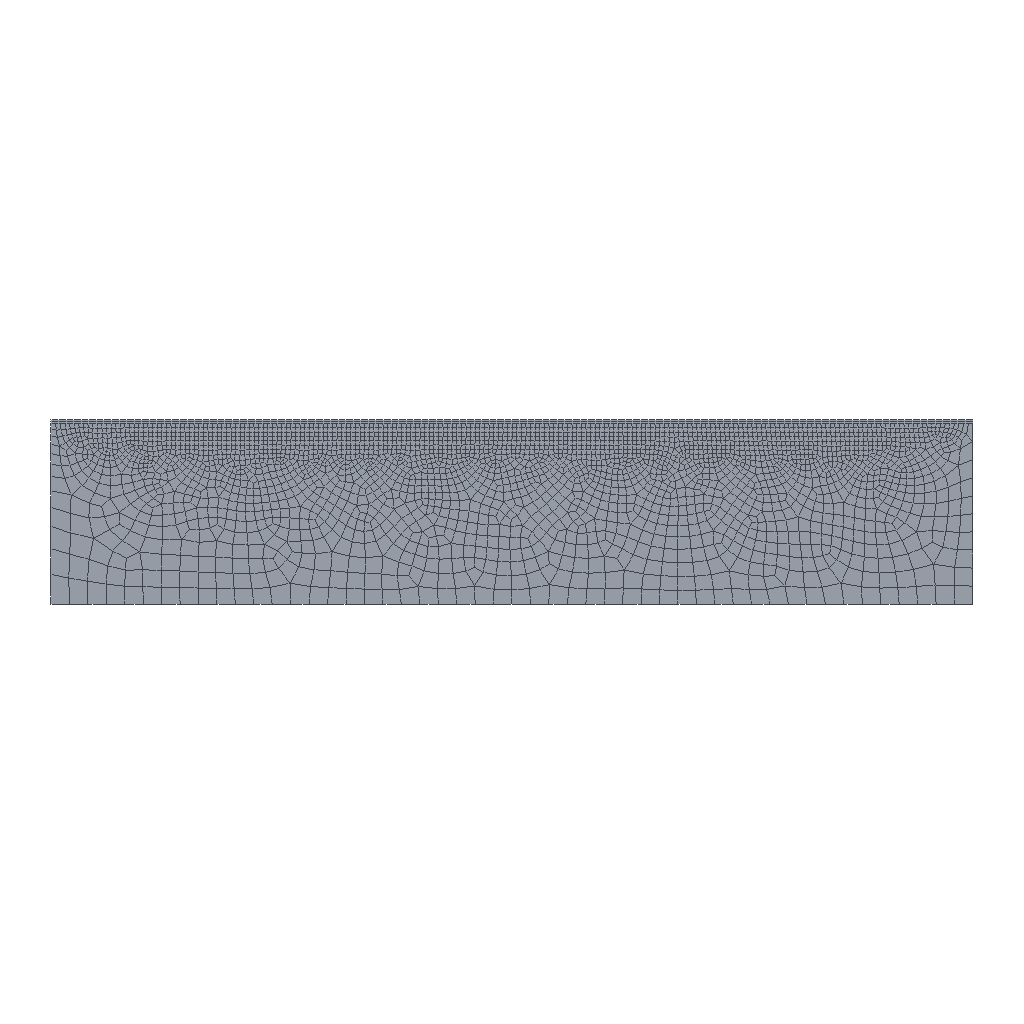Simulation study | abaqus
Set-up summary:
category,name,step,type,value,unit,region
solver,abaqus
solver,version,,,Abaqus/Standard 2020
units,not stated in the deck,,not stated
analysis,deck,,static,static
load_step,Step-1,Step-1,static
load_step,requested,,,1
mesh,nodes,,,3552
mesh,elements,,,3413
element_type,CPE4H,,plane,3413
load,load commands in deck,,count,1
bc,support commands in deck,,count,4
material,JIDI,,in results
material,MO,,in results
check,setup vs results,,match,"per instance, exact: element labels, types and connectivity; labels of the nodes the elements use; coordinates of those nodes at SINGLE_PRECISION in 1 of 1 instance(s)"
Abaqus input file, long lists of numbers shortened:
*Heading
** Job name: Job-1 Model name: Model-L1L2-2point5-L2H-50
** Generated by: Abaqus/CAE 2020
*Preprint, echo=NO, model=NO, history=NO, contact=NO
**
** PARTS
**
*Part, name=jidi
*Node
      1,           0., -0.2
      2,          50., -0.2
** (3550 more lines like these left out)
*Element, type=CPE4H
  1,   1,   7, 476, 406
  2,   7,   8, 477, 476
** (3411 more lines like these left out)
*Nset, nset=Set-2, generate
    1,  3552,     1
*Elset, elset=Set-2, generate
    1,  3413,     1
*Nset, nset=Set-3
    1,    2,    5,    6,    7,    8,    9,   10,   11,   12,   13,   14,   15,   16,   17,   18
   19,   20,   21,   22,   23,   24,   25,   26,   27,   28,   29,   30,   31,   32,   33,   34
** (195 more lines like these left out)
*Elset, elset=Set-3, generate
  401,  3413,     1
*Nset, nset=Set-4
   1,   2,   3,   4,   7,   8,   9,  10,  11,  12,  13,  14,  15,  16,  17,  18
  19,  20,  21,  22,  23,  24,  25,  26,  27,  28,  29,  30,  31,  32,  33,  34
** (36 more lines like these left out)
*Elset, elset=Set-4, generate
   1,  400,    1
** Section: Section-2
*Solid Section, elset=Set-4, material=jidi
,
** Section: Section-1
*Solid Section, elset=Set-3, material=mo
,
*End Part
**
**
** ASSEMBLY
**
*Assembly, name=Assembly
**
*Instance, name=jidi-1, part=jidi
*End Instance
**
*Nset, nset=Set-1, instance=jidi-1
   5,   6, 418, 419, 420, 421, 422, 423, 424, 425, 426, 427, 428, 429, 430, 431
 432, 433, 434, 435, 436, 437, 438, 439, 440, 441, 442, 443, 444, 445, 446, 447
** (2 more lines like these left out)
*Elset, elset=Set-1, instance=jidi-1
  405,  406,  407,  419,  436,  437,  438,  439,  456,  471,  472,  473,  490,  492,  509,  510
  511,  512,  515,  520,  525,  530,  531,  781,  782,  783,  786,  790,  801, 3227, 3232, 3245
** (2 more lines like these left out)
*Nset, nset=Set-2, instance=jidi-1
   5,   6, 418, 419, 420, 421, 422, 423, 424, 425, 426, 427, 428, 429, 430, 431
 432, 433, 434, 435, 436, 437, 438, 439, 440, 441, 442, 443, 444, 445, 446, 447
** (2 more lines like these left out)
*Elset, elset=Set-2, instance=jidi-1
  405,  406,  407,  419,  436,  437,  438,  439,  456,  471,  472,  473,  490,  492,  509,  510
  511,  512,  515,  520,  525,  530,  531,  781,  782,  783,  786,  790,  801, 3227, 3232, 3245
** (2 more lines like these left out)
*Nset, nset=Set-3, instance=jidi-1
   1,   4,   5, 406, 407, 408, 409, 410, 411, 412, 413, 414, 415, 416, 417
*Elset, elset=Set-3, instance=jidi-1
    1,  201,  466,  468,  469,  508,  511,  599,  600,  778,  779,  780,  958, 3271
*Nset, nset=Set-4, instance=jidi-1
   2,   3,   6, 206, 467, 468, 469, 470, 471, 472, 473, 474, 475
*Elset, elset=Set-4, instance=jidi-1
  200,  400,  406,  533,  802,  806, 1744, 2231, 2678, 2760, 3279, 3280
*Nset, nset=Set-5, instance=jidi-1
   1,   4,   5, 406, 407, 408, 409, 410, 411, 412, 413, 414, 415, 416, 417
*Elset, elset=Set-5, instance=jidi-1
    1,  201,  466,  468,  469,  508,  511,  599,  600,  778,  779,  780,  958, 3271
*Nset, nset=Set-6, instance=jidi-1
   2,   3,   6, 206, 467, 468, 469, 470, 471, 472, 473, 474, 475
*Elset, elset=Set-6, instance=jidi-1
  200,  400,  406,  533,  802,  806, 1744, 2231, 2678, 2760, 3279, 3280
*Nset, nset=Set-7, instance=jidi-1
   5,   6, 418, 419, 420, 421, 422, 423, 424, 425, 426, 427, 428, 429, 430, 431
 432, 433, 434, 435, 436, 437, 438, 439, 440, 441, 442, 443, 444, 445, 446, 447
** (2 more lines like these left out)
*Elset, elset=Set-7, instance=jidi-1
  405,  406,  407,  419,  436,  437,  438,  439,  456,  471,  472,  473,  490,  492,  509,  510
  511,  512,  515,  520,  525,  530,  531,  781,  782,  783,  786,  790,  801, 3227, 3232, 3245
** (2 more lines like these left out)
*Elset, elset=_m_Surf-1_S3, internal, instance=jidi-1, generate
 201,  400,    1
*Surface, type=ELEMENT, name=m_Surf-1
_m_Surf-1_S3, S3
*End Assembly
*Amplitude, name=Amp-1
             0.,              0.,              1.,              1.
**
** MATERIALS
**
*Material, name=jidi
*Elastic, moduli=LONG TERM
9000., 0.35
*Viscoelastic, frequency=PRONY
 0.1986,    0., 0.001
*Trs
1.,   4.5, 73.44
*Material, name=mo
*Elastic
 2.97, 0.495
**
** INTERACTION PROPERTIES
**
*Surface Interaction, name=IntProp-1
1.,
*Friction, slip tolerance=0.005
 0.1,
*Surface Behavior, pressure-overclosure=HARD
** ----------------------------------------------------------------
**
** STEP: Step-1
**
*Step, name=Step-1, nlgeom=YES, inc=10000
*Static, direct, stabilize, factor=0.0002, allsdtol=0, continue=NO
0.05, 10.,
**
** BOUNDARY CONDITIONS
**
** Name: BC-1 Type: 位移/转角
*Boundary
Set-7, 2, 2
** Name: BC-2 Type: 位移/转角
*Boundary
Set-5, 1, 1
Set-5, 2, 2
** Name: BC-3 Type: 位移/转角
*Boundary
Set-6, 1, 1, -0.5
**
** OUTPUT REQUESTS
**
*Restart, write, frequency=0
**
** FIELD OUTPUT: F-Output-1
**
*Output, field, frequency=10
*Node Output
CF, RF, U, V
*Element Output, directions=YES
E, LE, MISES, MISESMAX, PE, PEEQ, PEMAG, S
*Contact Output
CDISP, CSTRESS
**
** HISTORY OUTPUT: H-Output-1
**
*Output, history, variable=PRESELECT
*End Step
Results summary:
result,step,,completed,increments=200 time=10.0/10.0
result,analysis,,,static
result,last_loadstep,,,1
result,primary field,,,U
result,reaction total,,FX,-0.002298,model units
result,reaction total,,FY,0.000541,model units
result,reaction total,,FZ,0.0,model units